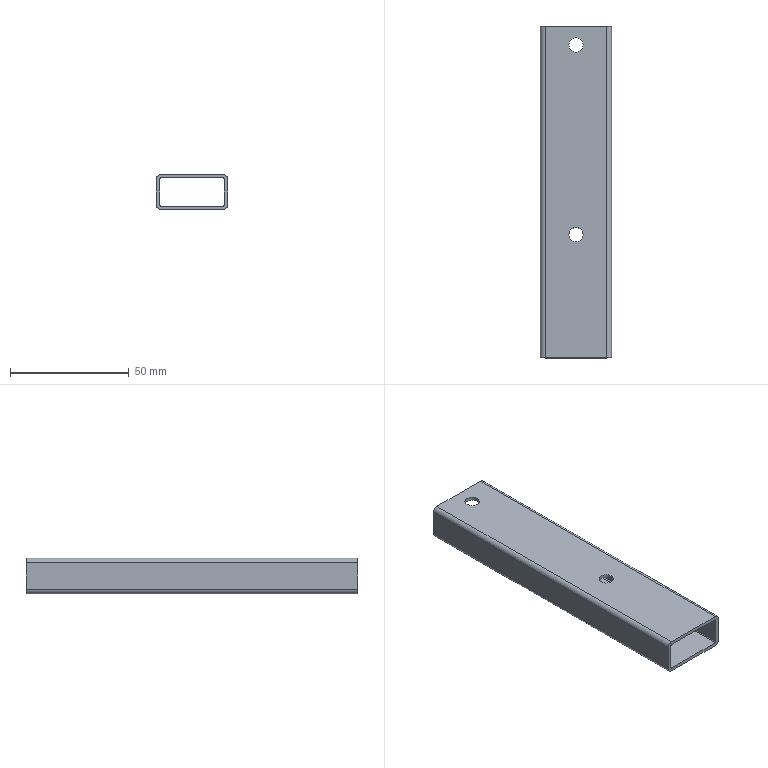Part | STEP file | 7471203 | 1 solid | 22 faces | box 30 x 140 x 15 mm | volume 17020 mm3 | cylinder 12 | plane 10 | commonest cylinder face diameters 1 x4 4 x4 6 x4